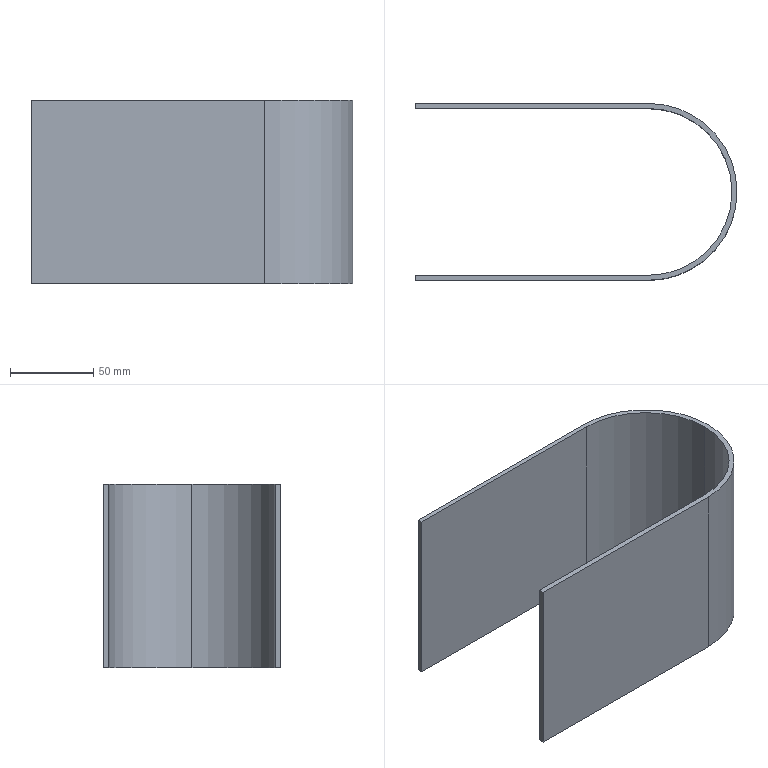Part | STEP file | 1 solid | 12 faces | box 193 x 106 x 110 mm | volume 145791 mm3 | plane 8 | cylinder 4 | commonest cylinder face diameters 100 x2 106 x2
STEP:
#1=CARTESIAN_POINT('',(0.,0.,0.));
#2=DIRECTION('',(0.,0.,1.));
#3=DIRECTION('',(1.,0.,0.));
#4=AXIS2_PLACEMENT_3D('',#1,#2,#3);
#5=CARTESIAN_POINT('',(27.634,-77.901,0.));
#6=VERTEX_POINT('',#5);
#7=CARTESIAN_POINT('',(80.634,-24.901,0.));
#8=VERTEX_POINT('',#7);
#9=CARTESIAN_POINT('',(27.634,-24.901,0.));
#10=DIRECTION('',(0.,0.,1.));
#11=DIRECTION('',(1.,0.,0.));
#12=AXIS2_PLACEMENT_3D('',#9,#10,#11);
#13=CIRCLE('',#12,53.);
#14=CARTESIAN_POINT('',(27.634,-24.901,0.));
#15=DIRECTION('',(0.,0.,1.));
#16=DIRECTION('',(1.,0.,0.));
#17=AXIS2_PLACEMENT_3D('',#14,#15,#16);
#18=CYLINDRICAL_SURFACE('',#17,53.);
#19=CARTESIAN_POINT('',(0.,0.));
#20=DIRECTION('',(1.,0.));
#21=VECTOR('',#20,1.);
#22=LINE('',#19,#21);
#23=(GEOMETRIC_REPRESENTATION_CONTEXT(2)PARAMETRIC_REPRESENTATION_CONTEXT()REPRESENTATION_CONTEXT('',''));
#24=DEFINITIONAL_REPRESENTATION('',(#22),#23);
#25=PCURVE('',#18,#24);
#26=CARTESIAN_POINT('',(-12.03,-24.901,0.));
#27=DIRECTION('',(0.,0.,1.));
#28=DIRECTION('',(1.,0.,0.));
#29=AXIS2_PLACEMENT_3D('',#26,#27,#28);
#30=PLANE('',#29);
#31=CARTESIAN_POINT('',(39.665,0.));
#32=DIRECTION('',(1.,0.));
#33=AXIS2_PLACEMENT_2D('',#31,#32);
#34=CIRCLE('',#33,53.);
#35=(GEOMETRIC_REPRESENTATION_CONTEXT(2)PARAMETRIC_REPRESENTATION_CONTEXT()REPRESENTATION_CONTEXT('',''));
#36=DEFINITIONAL_REPRESENTATION('',(#34),#35);
#37=PCURVE('',#30,#36);
#38=SURFACE_CURVE('',#13,(#25,#37),.PCURVE_S1.);
#39=EDGE_CURVE('',#6,#8,#38,.T.);
#40=ORIENTED_EDGE('',*,*,#39,.T.);
#41=CARTESIAN_POINT('',(80.634,-24.901,110.));
#42=VERTEX_POINT('',#41);
#43=CARTESIAN_POINT('',(80.634,-24.901,0.));
#44=DIRECTION('',(0.,0.,1.));
#45=VECTOR('',#44,1.);
#46=LINE('',#43,#45);
#47=CARTESIAN_POINT('',(6.283,0.));
#48=DIRECTION('',(0.,1.));
#49=VECTOR('',#48,1.);
#50=LINE('',#47,#49);
#51=(GEOMETRIC_REPRESENTATION_CONTEXT(2)PARAMETRIC_REPRESENTATION_CONTEXT()REPRESENTATION_CONTEXT('',''));
#52=DEFINITIONAL_REPRESENTATION('',(#50),#51);
#53=PCURVE('',#18,#52);
#54=CARTESIAN_POINT('',(27.634,-24.901,0.));
#55=DIRECTION('',(0.,0.,1.));
#56=DIRECTION('',(1.,0.,0.));
#57=AXIS2_PLACEMENT_3D('',#54,#55,#56);
#58=CYLINDRICAL_SURFACE('',#57,53.);
#59=CARTESIAN_POINT('',(0.,0.));
#60=DIRECTION('',(0.,1.));
#61=VECTOR('',#60,1.);
#62=LINE('',#59,#61);
#63=(GEOMETRIC_REPRESENTATION_CONTEXT(2)PARAMETRIC_REPRESENTATION_CONTEXT()REPRESENTATION_CONTEXT('',''));
#64=DEFINITIONAL_REPRESENTATION('',(#62),#63);
#65=PCURVE('',#58,#64);
#66=SURFACE_CURVE('',#46,(#53,#65),.PCURVE_S1.);
#67=EDGE_CURVE('',#8,#42,#66,.T.);
#68=ORIENTED_EDGE('',*,*,#67,.T.);
#69=CARTESIAN_POINT('',(27.634,-77.901,110.));
#70=VERTEX_POINT('',#69);
#71=CARTESIAN_POINT('',(27.634,-24.901,110.));
#72=DIRECTION('',(0.,0.,-1.));
#73=DIRECTION('',(1.,0.,0.));
#74=AXIS2_PLACEMENT_3D('',#71,#72,#73);
#75=CIRCLE('',#74,53.);
#76=CARTESIAN_POINT('',(6.283,110.));
#77=DIRECTION('',(-1.,0.));
#78=VECTOR('',#77,1.);
#79=LINE('',#76,#78);
#80=(GEOMETRIC_REPRESENTATION_CONTEXT(2)PARAMETRIC_REPRESENTATION_CONTEXT()REPRESENTATION_CONTEXT('',''));
#81=DEFINITIONAL_REPRESENTATION('',(#79),#80);
#82=PCURVE('',#18,#81);
#83=CARTESIAN_POINT('',(-12.03,-24.901,110.));
#84=DIRECTION('',(0.,0.,1.));
#85=DIRECTION('',(1.,0.,0.));
#86=AXIS2_PLACEMENT_3D('',#83,#84,#85);
#87=PLANE('',#86);
#88=CARTESIAN_POINT('',(92.665,0.));
#89=CARTESIAN_POINT('',(92.665,-91.799));
#90=CARTESIAN_POINT('',(13.165,-45.899));
#91=CARTESIAN_POINT('',(-66.335,0.));
#92=CARTESIAN_POINT('',(13.165,45.899));
#93=CARTESIAN_POINT('',(92.665,91.799));
#94=CARTESIAN_POINT('',(92.665,0.));
#95=(BOUNDED_CURVE()B_SPLINE_CURVE(2,(#88,#89,#90,#91,#92,#93,#94),.UNSPECIFIED.,.T.,.F.)B_SPLINE_CURVE_WITH_KNOTS((1,2,2,2,2,1),(-2.094,0.,2.094,4.189,6.283,8.378),.UNSPECIFIED.)CURVE()GEOMETRIC_REPRESENTATION_ITEM()RATIONAL_B_SPLINE_CURVE((1.,0.5,1.,0.5,1.,0.5,1.))REPRESENTATION_ITEM(''));
#96=(GEOMETRIC_REPRESENTATION_CONTEXT(2)PARAMETRIC_REPRESENTATION_CONTEXT()REPRESENTATION_CONTEXT('',''));
#97=DEFINITIONAL_REPRESENTATION('',(#95),#96);
#98=PCURVE('',#87,#97);
#99=SURFACE_CURVE('',#75,(#82,#98),.PCURVE_S1.);
#100=EDGE_CURVE('',#42,#70,#99,.T.);
#101=ORIENTED_EDGE('',*,*,#100,.T.);
#102=CARTESIAN_POINT('',(27.634,-77.901,0.));
#103=DIRECTION('',(0.,0.,-1.));
#104=VECTOR('',#103,1.);
#105=LINE('',#102,#104);
#106=CARTESIAN_POINT('',(4.712,0.));
#107=DIRECTION('',(0.,-1.));
#108=VECTOR('',#107,1.);
#109=LINE('',#106,#108);
#110=(GEOMETRIC_REPRESENTATION_CONTEXT(2)PARAMETRIC_REPRESENTATION_CONTEXT()REPRESENTATION_CONTEXT('',''));
#111=DEFINITIONAL_REPRESENTATION('',(#109),#110);
#112=PCURVE('',#18,#111);
#113=CARTESIAN_POINT('',(-112.366,-77.901,0.));
#114=DIRECTION('',(0.,-1.,0.));
#115=DIRECTION('',(1.,0.,0.));
#116=AXIS2_PLACEMENT_3D('',#113,#114,#115);
#117=PLANE('',#116);
#118=CARTESIAN_POINT('',(140.,0.));
#119=DIRECTION('',(0.,-1.));
#120=VECTOR('',#119,1.);
#121=LINE('',#118,#120);
#122=(GEOMETRIC_REPRESENTATION_CONTEXT(2)PARAMETRIC_REPRESENTATION_CONTEXT()REPRESENTATION_CONTEXT('',''));
#123=DEFINITIONAL_REPRESENTATION('',(#121),#122);
#124=PCURVE('',#117,#123);
#125=SURFACE_CURVE('',#105,(#112,#124),.PCURVE_S1.);
#126=EDGE_CURVE('',#70,#6,#125,.T.);
#127=ORIENTED_EDGE('',*,*,#126,.T.);
#128=EDGE_LOOP('',(#40,#68,#101,#127));
#129=FACE_BOUND('',#128,.T.);
#130=ADVANCED_FACE('',(#129),#18,.T.);
#131=CARTESIAN_POINT('',(27.634,25.099,0.));
#132=VERTEX_POINT('',#131);
#133=CARTESIAN_POINT('',(27.634,25.099,110.));
#134=VERTEX_POINT('',#133);
#135=CARTESIAN_POINT('',(27.634,25.099,0.));
#136=DIRECTION('',(0.,0.,1.));
#137=VECTOR('',#136,1.);
#138=LINE('',#135,#137);
#139=CARTESIAN_POINT('',(27.634,-24.901,0.));
#140=DIRECTION('',(0.,0.,1.));
#141=DIRECTION('',(1.,0.,0.));
#142=AXIS2_PLACEMENT_3D('',#139,#140,#141);
#143=CYLINDRICAL_SURFACE('',#142,50.);
#144=CARTESIAN_POINT('',(1.571,0.));
#145=DIRECTION('',(0.,1.));
#146=VECTOR('',#145,1.);
#147=LINE('',#144,#146);
#148=(GEOMETRIC_REPRESENTATION_CONTEXT(2)PARAMETRIC_REPRESENTATION_CONTEXT()REPRESENTATION_CONTEXT('',''));
#149=DEFINITIONAL_REPRESENTATION('',(#147),#148);
#150=PCURVE('',#143,#149);
#151=CARTESIAN_POINT('',(-112.366,25.099,0.));
#152=DIRECTION('',(0.,-1.,0.));
#153=DIRECTION('',(0.,0.,-1.));
#154=AXIS2_PLACEMENT_3D('',#151,#152,#153);
#155=PLANE('',#154);
#156=CARTESIAN_POINT('',(0.,140.));
#157=DIRECTION('',(-1.,0.));
#158=VECTOR('',#157,1.);
#159=LINE('',#156,#158);
#160=(GEOMETRIC_REPRESENTATION_CONTEXT(2)PARAMETRIC_REPRESENTATION_CONTEXT()REPRESENTATION_CONTEXT('',''));
#161=DEFINITIONAL_REPRESENTATION('',(#159),#160);
#162=PCURVE('',#155,#161);
#163=SURFACE_CURVE('',#138,(#150,#162),.PCURVE_S1.);
#164=EDGE_CURVE('',#132,#134,#163,.T.);
#165=ORIENTED_EDGE('',*,*,#164,.T.);
#166=CARTESIAN_POINT('',(77.634,-24.901,110.));
#167=VERTEX_POINT('',#166);
#168=CARTESIAN_POINT('',(27.634,-24.901,110.));
#169=DIRECTION('',(0.,0.,-1.));
#170=DIRECTION('',(1.,0.,0.));
#171=AXIS2_PLACEMENT_3D('',#168,#169,#170);
#172=CIRCLE('',#171,50.);
#173=CARTESIAN_POINT('',(6.283,110.));
#174=DIRECTION('',(-1.,0.));
#175=VECTOR('',#174,1.);
#176=LINE('',#173,#175);
#177=(GEOMETRIC_REPRESENTATION_CONTEXT(2)PARAMETRIC_REPRESENTATION_CONTEXT()REPRESENTATION_CONTEXT('',''));
#178=DEFINITIONAL_REPRESENTATION('',(#176),#177);
#179=PCURVE('',#143,#178);
#180=CARTESIAN_POINT('',(89.665,0.));
#181=CARTESIAN_POINT('',(89.665,-86.603));
#182=CARTESIAN_POINT('',(14.665,-43.301));
#183=CARTESIAN_POINT('',(-60.335,0.));
#184=CARTESIAN_POINT('',(14.665,43.301));
#185=CARTESIAN_POINT('',(89.665,86.603));
#186=CARTESIAN_POINT('',(89.665,0.));
#187=(BOUNDED_CURVE()B_SPLINE_CURVE(2,(#180,#181,#182,#183,#184,#185,#186),.UNSPECIFIED.,.T.,.F.)B_SPLINE_CURVE_WITH_KNOTS((1,2,2,2,2,1),(-2.094,0.,2.094,4.189,6.283,8.378),.UNSPECIFIED.)CURVE()GEOMETRIC_REPRESENTATION_ITEM()RATIONAL_B_SPLINE_CURVE((1.,0.5,1.,0.5,1.,0.5,1.))REPRESENTATION_ITEM(''));
#188=(GEOMETRIC_REPRESENTATION_CONTEXT(2)PARAMETRIC_REPRESENTATION_CONTEXT()REPRESENTATION_CONTEXT('',''));
#189=DEFINITIONAL_REPRESENTATION('',(#187),#188);
#190=PCURVE('',#87,#189);
#191=SURFACE_CURVE('',#172,(#179,#190),.PCURVE_S1.);
#192=EDGE_CURVE('',#134,#167,#191,.T.);
#193=ORIENTED_EDGE('',*,*,#192,.T.);
#194=CARTESIAN_POINT('',(77.634,-24.901,0.));
#195=VERTEX_POINT('',#194);
#196=CARTESIAN_POINT('',(77.634,-24.901,0.));
#197=DIRECTION('',(0.,0.,1.));
#198=VECTOR('',#197,1.);
#199=LINE('',#196,#198);
#200=CARTESIAN_POINT('',(0.,0.));
#201=DIRECTION('',(0.,1.));
#202=VECTOR('',#201,1.);
#203=LINE('',#200,#202);
#204=(GEOMETRIC_REPRESENTATION_CONTEXT(2)PARAMETRIC_REPRESENTATION_CONTEXT()REPRESENTATION_CONTEXT('',''));
#205=DEFINITIONAL_REPRESENTATION('',(#203),#204);
#206=PCURVE('',#143,#205);
#207=CARTESIAN_POINT('',(27.634,-24.901,0.));
#208=DIRECTION('',(0.,0.,1.));
#209=DIRECTION('',(1.,0.,0.));
#210=AXIS2_PLACEMENT_3D('',#207,#208,#209);
#211=CYLINDRICAL_SURFACE('',#210,50.);
#212=CARTESIAN_POINT('',(6.283,0.));
#213=DIRECTION('',(0.,1.));
#214=VECTOR('',#213,1.);
#215=LINE('',#212,#214);
#216=(GEOMETRIC_REPRESENTATION_CONTEXT(2)PARAMETRIC_REPRESENTATION_CONTEXT()REPRESENTATION_CONTEXT('',''));
#217=DEFINITIONAL_REPRESENTATION('',(#215),#216);
#218=PCURVE('',#211,#217);
#219=SURFACE_CURVE('',#199,(#206,#218),.PCURVE_S1.);
#220=EDGE_CURVE('',#195,#167,#219,.T.);
#221=ORIENTED_EDGE('',*,*,#220,.F.);
#222=CARTESIAN_POINT('',(27.634,-24.901,0.));
#223=DIRECTION('',(0.,0.,-1.));
#224=DIRECTION('',(1.,0.,0.));
#225=AXIS2_PLACEMENT_3D('',#222,#223,#224);
#226=CIRCLE('',#225,50.);
#227=CARTESIAN_POINT('',(6.283,0.));
#228=DIRECTION('',(-1.,0.));
#229=VECTOR('',#228,1.);
#230=LINE('',#227,#229);
#231=(GEOMETRIC_REPRESENTATION_CONTEXT(2)PARAMETRIC_REPRESENTATION_CONTEXT()REPRESENTATION_CONTEXT('',''));
#232=DEFINITIONAL_REPRESENTATION('',(#230),#231);
#233=PCURVE('',#143,#232);
#234=CARTESIAN_POINT('',(89.665,0.));
#235=CARTESIAN_POINT('',(89.665,-86.603));
#236=CARTESIAN_POINT('',(14.665,-43.301));
#237=CARTESIAN_POINT('',(-60.335,0.));
#238=CARTESIAN_POINT('',(14.665,43.301));
#239=CARTESIAN_POINT('',(89.665,86.603));
#240=CARTESIAN_POINT('',(89.665,0.));
#241=(BOUNDED_CURVE()B_SPLINE_CURVE(2,(#234,#235,#236,#237,#238,#239,#240),.UNSPECIFIED.,.T.,.F.)B_SPLINE_CURVE_WITH_KNOTS((1,2,2,2,2,1),(-2.094,0.,2.094,4.189,6.283,8.378),.UNSPECIFIED.)CURVE()GEOMETRIC_REPRESENTATION_ITEM()RATIONAL_B_SPLINE_CURVE((1.,0.5,1.,0.5,1.,0.5,1.))REPRESENTATION_ITEM(''));
#242=(GEOMETRIC_REPRESENTATION_CONTEXT(2)PARAMETRIC_REPRESENTATION_CONTEXT()REPRESENTATION_CONTEXT('',''));
#243=DEFINITIONAL_REPRESENTATION('',(#241),#242);
#244=PCURVE('',#30,#243);
#245=SURFACE_CURVE('',#226,(#233,#244),.PCURVE_S1.);
#246=EDGE_CURVE('',#132,#195,#245,.T.);
#247=ORIENTED_EDGE('',*,*,#246,.F.);
#248=EDGE_LOOP('',(#165,#193,#221,#247));
#249=FACE_BOUND('',#248,.F.);
#250=ADVANCED_FACE('',(#249),#143,.F.);
#251=ORIENTED_EDGE('',*,*,#67,.F.);
#252=CARTESIAN_POINT('',(27.634,28.099,0.));
#253=VERTEX_POINT('',#252);
#254=CARTESIAN_POINT('',(27.634,-24.901,0.));
#255=DIRECTION('',(0.,0.,1.));
#256=DIRECTION('',(1.,0.,0.));
#257=AXIS2_PLACEMENT_3D('',#254,#255,#256);
#258=CIRCLE('',#257,53.);
#259=CARTESIAN_POINT('',(0.,0.));
#260=DIRECTION('',(1.,0.));
#261=VECTOR('',#260,1.);
#262=LINE('',#259,#261);
#263=(GEOMETRIC_REPRESENTATION_CONTEXT(2)PARAMETRIC_REPRESENTATION_CONTEXT()REPRESENTATION_CONTEXT('',''));
#264=DEFINITIONAL_REPRESENTATION('',(#262),#263);
#265=PCURVE('',#58,#264);
#266=CARTESIAN_POINT('',(39.665,0.));
#267=DIRECTION('',(1.,0.));
#268=AXIS2_PLACEMENT_2D('',#266,#267);
#269=CIRCLE('',#268,53.);
#270=(GEOMETRIC_REPRESENTATION_CONTEXT(2)PARAMETRIC_REPRESENTATION_CONTEXT()REPRESENTATION_CONTEXT('',''));
#271=DEFINITIONAL_REPRESENTATION('',(#269),#270);
#272=PCURVE('',#30,#271);
#273=SURFACE_CURVE('',#258,(#265,#272),.PCURVE_S1.);
#274=EDGE_CURVE('',#8,#253,#273,.T.);
#275=ORIENTED_EDGE('',*,*,#274,.T.);
#276=CARTESIAN_POINT('',(27.634,28.099,110.));
#277=VERTEX_POINT('',#276);
#278=CARTESIAN_POINT('',(27.634,28.099,0.));
#279=DIRECTION('',(0.,0.,1.));
#280=VECTOR('',#279,1.);
#281=LINE('',#278,#280);
#282=CARTESIAN_POINT('',(1.571,0.));
#283=DIRECTION('',(0.,1.));
#284=VECTOR('',#283,1.);
#285=LINE('',#282,#284);
#286=(GEOMETRIC_REPRESENTATION_CONTEXT(2)PARAMETRIC_REPRESENTATION_CONTEXT()REPRESENTATION_CONTEXT('',''));
#287=DEFINITIONAL_REPRESENTATION('',(#285),#286);
#288=PCURVE('',#58,#287);
#289=CARTESIAN_POINT('',(27.634,28.099,0.));
#290=DIRECTION('',(0.,1.,0.));
#291=DIRECTION('',(-1.,0.,0.));
#292=AXIS2_PLACEMENT_3D('',#289,#290,#291);
#293=PLANE('',#292);
#294=CARTESIAN_POINT('',(0.,0.));
#295=DIRECTION('',(0.,1.));
#296=VECTOR('',#295,1.);
#297=LINE('',#294,#296);
#298=(GEOMETRIC_REPRESENTATION_CONTEXT(2)PARAMETRIC_REPRESENTATION_CONTEXT()REPRESENTATION_CONTEXT('',''));
#299=DEFINITIONAL_REPRESENTATION('',(#297),#298);
#300=PCURVE('',#293,#299);
#301=SURFACE_CURVE('',#281,(#288,#300),.PCURVE_S1.);
#302=EDGE_CURVE('',#253,#277,#301,.T.);
#303=ORIENTED_EDGE('',*,*,#302,.T.);
#304=CARTESIAN_POINT('',(27.634,-24.901,110.));
#305=DIRECTION('',(0.,0.,-1.));
#306=DIRECTION('',(1.,0.,0.));
#307=AXIS2_PLACEMENT_3D('',#304,#305,#306);
#308=CIRCLE('',#307,53.);
#309=CARTESIAN_POINT('',(6.283,110.));
#310=DIRECTION('',(-1.,0.));
#311=VECTOR('',#310,1.);
#312=LINE('',#309,#311);
#313=(GEOMETRIC_REPRESENTATION_CONTEXT(2)PARAMETRIC_REPRESENTATION_CONTEXT()REPRESENTATION_CONTEXT('',''));
#314=DEFINITIONAL_REPRESENTATION('',(#312),#313);
#315=PCURVE('',#58,#314);
#316=CARTESIAN_POINT('',(92.665,0.));
#317=CARTESIAN_POINT('',(92.665,-91.799));
#318=CARTESIAN_POINT('',(13.165,-45.899));
#319=CARTESIAN_POINT('',(-66.335,0.));
#320=CARTESIAN_POINT('',(13.165,45.899));
#321=CARTESIAN_POINT('',(92.665,91.799));
#322=CARTESIAN_POINT('',(92.665,0.));
#323=(BOUNDED_CURVE()B_SPLINE_CURVE(2,(#316,#317,#318,#319,#320,#321,#322),.UNSPECIFIED.,.T.,.F.)B_SPLINE_CURVE_WITH_KNOTS((1,2,2,2,2,1),(-2.094,0.,2.094,4.189,6.283,8.378),.UNSPECIFIED.)CURVE()GEOMETRIC_REPRESENTATION_ITEM()RATIONAL_B_SPLINE_CURVE((1.,0.5,1.,0.5,1.,0.5,1.))REPRESENTATION_ITEM(''));
#324=(GEOMETRIC_REPRESENTATION_CONTEXT(2)PARAMETRIC_REPRESENTATION_CONTEXT()REPRESENTATION_CONTEXT('',''));
#325=DEFINITIONAL_REPRESENTATION('',(#323),#324);
#326=PCURVE('',#87,#325);
#327=SURFACE_CURVE('',#308,(#315,#326),.PCURVE_S1.);
#328=EDGE_CURVE('',#277,#42,#327,.T.);
#329=ORIENTED_EDGE('',*,*,#328,.T.);
#330=EDGE_LOOP('',(#251,#275,#303,#329));
#331=FACE_BOUND('',#330,.T.);
#332=ADVANCED_FACE('',(#331),#58,.T.);
#333=CARTESIAN_POINT('',(-112.366,-77.901,110.));
#334=VERTEX_POINT('',#333);
#335=CARTESIAN_POINT('',(-112.366,-77.901,110.));
#336=DIRECTION('',(-1.,0.,0.));
#337=VECTOR('',#336,1.);
#338=LINE('',#335,#337);
#339=CARTESIAN_POINT('',(0.,110.));
#340=DIRECTION('',(-1.,0.));
#341=VECTOR('',#340,1.);
#342=LINE('',#339,#341);
#343=(GEOMETRIC_REPRESENTATION_CONTEXT(2)PARAMETRIC_REPRESENTATION_CONTEXT()REPRESENTATION_CONTEXT('',''));
#344=DEFINITIONAL_REPRESENTATION('',(#342),#343);
#345=PCURVE('',#117,#344);
#346=CARTESIAN_POINT('',(-100.335,-53.));
#347=DIRECTION('',(-1.,0.));
#348=VECTOR('',#347,1.);
#349=LINE('',#346,#348);
#350=(GEOMETRIC_REPRESENTATION_CONTEXT(2)PARAMETRIC_REPRESENTATION_CONTEXT()REPRESENTATION_CONTEXT('',''));
#351=DEFINITIONAL_REPRESENTATION('',(#349),#350);
#352=PCURVE('',#87,#351);
#353=SURFACE_CURVE('',#338,(#345,#352),.PCURVE_S1.);
#354=EDGE_CURVE('',#70,#334,#353,.T.);
#355=ORIENTED_EDGE('',*,*,#354,.T.);
#356=CARTESIAN_POINT('',(-112.366,-77.901,0.));
#357=VERTEX_POINT('',#356);
#358=CARTESIAN_POINT('',(-112.366,-77.901,0.));
#359=DIRECTION('',(0.,0.,-1.));
#360=VECTOR('',#359,1.);
#361=LINE('',#358,#360);
#362=CARTESIAN_POINT('',(0.,0.));
#363=DIRECTION('',(0.,-1.));
#364=VECTOR('',#363,1.);
#365=LINE('',#362,#364);
#366=(GEOMETRIC_REPRESENTATION_CONTEXT(2)PARAMETRIC_REPRESENTATION_CONTEXT()REPRESENTATION_CONTEXT('',''));
#367=DEFINITIONAL_REPRESENTATION('',(#365),#366);
#368=PCURVE('',#117,#367);
#369=CARTESIAN_POINT('',(-112.366,-74.901,0.));
#370=DIRECTION('',(-1.,0.,0.));
#371=DIRECTION('',(0.,0.,1.));
#372=AXIS2_PLACEMENT_3D('',#369,#370,#371);
#373=PLANE('',#372);
#374=CARTESIAN_POINT('',(0.,-3.));
#375=DIRECTION('',(-1.,0.));
#376=VECTOR('',#375,1.);
#377=LINE('',#374,#376);
#378=(GEOMETRIC_REPRESENTATION_CONTEXT(2)PARAMETRIC_REPRESENTATION_CONTEXT()REPRESENTATION_CONTEXT('',''));
#379=DEFINITIONAL_REPRESENTATION('',(#377),#378);
#380=PCURVE('',#373,#379);
#381=SURFACE_CURVE('',#361,(#368,#380),.PCURVE_S1.);
#382=EDGE_CURVE('',#334,#357,#381,.T.);
#383=ORIENTED_EDGE('',*,*,#382,.T.);
#384=CARTESIAN_POINT('',(-112.366,-77.901,0.));
#385=DIRECTION('',(1.,0.,0.));
#386=VECTOR('',#385,1.);
#387=LINE('',#384,#386);
#388=CARTESIAN_POINT('',(0.,0.));
#389=DIRECTION('',(1.,0.));
#390=VECTOR('',#389,1.);
#391=LINE('',#388,#390);
#392=(GEOMETRIC_REPRESENTATION_CONTEXT(2)PARAMETRIC_REPRESENTATION_CONTEXT()REPRESENTATION_CONTEXT('',''));
#393=DEFINITIONAL_REPRESENTATION('',(#391),#392);
#394=PCURVE('',#117,#393);
#395=CARTESIAN_POINT('',(-100.335,-53.));
#396=DIRECTION('',(1.,0.));
#397=VECTOR('',#396,1.);
#398=LINE('',#395,#397);
#399=(GEOMETRIC_REPRESENTATION_CONTEXT(2)PARAMETRIC_REPRESENTATION_CONTEXT()REPRESENTATION_CONTEXT('',''));
#400=DEFINITIONAL_REPRESENTATION('',(#398),#399);
#401=PCURVE('',#30,#400);
#402=SURFACE_CURVE('',#387,(#394,#401),.PCURVE_S1.);
#403=EDGE_CURVE('',#357,#6,#402,.T.);
#404=ORIENTED_EDGE('',*,*,#403,.T.);
#405=ORIENTED_EDGE('',*,*,#126,.F.);
#406=EDGE_LOOP('',(#355,#383,#404,#405));
#407=FACE_BOUND('',#406,.T.);
#408=ADVANCED_FACE('',(#407),#117,.T.);
#409=CARTESIAN_POINT('',(-112.366,28.099,110.));
#410=VERTEX_POINT('',#409);
#411=CARTESIAN_POINT('',(-12.03,28.099,110.));
#412=DIRECTION('',(-1.,0.,0.));
#413=VECTOR('',#412,1.);
#414=LINE('',#411,#413);
#415=CARTESIAN_POINT('',(0.,53.));
#416=DIRECTION('',(-1.,0.));
#417=VECTOR('',#416,1.);
#418=LINE('',#415,#417);
#419=(GEOMETRIC_REPRESENTATION_CONTEXT(2)PARAMETRIC_REPRESENTATION_CONTEXT()REPRESENTATION_CONTEXT('',''));
#420=DEFINITIONAL_REPRESENTATION('',(#418),#419);
#421=PCURVE('',#87,#420);
#422=CARTESIAN_POINT('',(39.665,110.));
#423=DIRECTION('',(1.,0.));
#424=VECTOR('',#423,1.);
#425=LINE('',#422,#424);
#426=(GEOMETRIC_REPRESENTATION_CONTEXT(2)PARAMETRIC_REPRESENTATION_CONTEXT()REPRESENTATION_CONTEXT('',''));
#427=DEFINITIONAL_REPRESENTATION('',(#425),#426);
#428=PCURVE('',#293,#427);
#429=SURFACE_CURVE('',#414,(#421,#428),.PCURVE_S1.);
#430=EDGE_CURVE('',#277,#410,#429,.T.);
#431=ORIENTED_EDGE('',*,*,#430,.T.);
#432=CARTESIAN_POINT('',(-112.366,25.099,110.));
#433=VERTEX_POINT('',#432);
#434=CARTESIAN_POINT('',(-112.366,-24.901,110.));
#435=DIRECTION('',(0.,-1.,0.));
#436=VECTOR('',#435,1.);
#437=LINE('',#434,#436);
#438=CARTESIAN_POINT('',(-100.335,0.));
#439=DIRECTION('',(0.,-1.));
#440=VECTOR('',#439,1.);
#441=LINE('',#438,#440);
#442=(GEOMETRIC_REPRESENTATION_CONTEXT(2)PARAMETRIC_REPRESENTATION_CONTEXT()REPRESENTATION_CONTEXT('',''));
#443=DEFINITIONAL_REPRESENTATION('',(#441),#442);
#444=PCURVE('',#87,#443);
#445=CARTESIAN_POINT('',(-112.366,28.099,0.));
#446=DIRECTION('',(-1.,0.,0.));
#447=DIRECTION('',(0.,0.,1.));
#448=AXIS2_PLACEMENT_3D('',#445,#446,#447);
#449=PLANE('',#448);
#450=CARTESIAN_POINT('',(110.,-53.));
#451=DIRECTION('',(0.,-1.));
#452=VECTOR('',#451,1.);
#453=LINE('',#450,#452);
#454=(GEOMETRIC_REPRESENTATION_CONTEXT(2)PARAMETRIC_REPRESENTATION_CONTEXT()REPRESENTATION_CONTEXT('',''));
#455=DEFINITIONAL_REPRESENTATION('',(#453),#454);
#456=PCURVE('',#449,#455);
#457=SURFACE_CURVE('',#437,(#444,#456),.PCURVE_S1.);
#458=EDGE_CURVE('',#410,#433,#457,.T.);
#459=ORIENTED_EDGE('',*,*,#458,.T.);
#460=CARTESIAN_POINT('',(-12.03,25.099,110.));
#461=DIRECTION('',(1.,0.,0.));
#462=VECTOR('',#461,1.);
#463=LINE('',#460,#462);
#464=CARTESIAN_POINT('',(0.,50.));
#465=DIRECTION('',(1.,0.));
#466=VECTOR('',#465,1.);
#467=LINE('',#464,#466);
#468=(GEOMETRIC_REPRESENTATION_CONTEXT(2)PARAMETRIC_REPRESENTATION_CONTEXT()REPRESENTATION_CONTEXT('',''));
#469=DEFINITIONAL_REPRESENTATION('',(#467),#468);
#470=PCURVE('',#87,#469);
#471=CARTESIAN_POINT('',(-110.,100.335));
#472=DIRECTION('',(0.,1.));
#473=VECTOR('',#472,1.);
#474=LINE('',#471,#473);
#475=(GEOMETRIC_REPRESENTATION_CONTEXT(2)PARAMETRIC_REPRESENTATION_CONTEXT()REPRESENTATION_CONTEXT('',''));
#476=DEFINITIONAL_REPRESENTATION('',(#474),#475);
#477=PCURVE('',#155,#476);
#478=SURFACE_CURVE('',#463,(#470,#477),.PCURVE_S1.);
#479=EDGE_CURVE('',#433,#134,#478,.T.);
#480=ORIENTED_EDGE('',*,*,#479,.T.);
#481=ORIENTED_EDGE('',*,*,#192,.T.);
#482=CARTESIAN_POINT('',(27.634,-74.901,110.));
#483=VERTEX_POINT('',#482);
#484=CARTESIAN_POINT('',(27.634,-24.901,110.));
#485=DIRECTION('',(0.,0.,-1.));
#486=DIRECTION('',(1.,0.,0.));
#487=AXIS2_PLACEMENT_3D('',#484,#485,#486);
#488=CIRCLE('',#487,50.);
#489=CARTESIAN_POINT('',(89.665,0.));
#490=CARTESIAN_POINT('',(89.665,-86.603));
#491=CARTESIAN_POINT('',(14.665,-43.301));
#492=CARTESIAN_POINT('',(-60.335,0.));
#493=CARTESIAN_POINT('',(14.665,43.301));
#494=CARTESIAN_POINT('',(89.665,86.603));
#495=CARTESIAN_POINT('',(89.665,0.));
#496=(BOUNDED_CURVE()B_SPLINE_CURVE(2,(#489,#490,#491,#492,#493,#494,#495),.UNSPECIFIED.,.T.,.F.)B_SPLINE_CURVE_WITH_KNOTS((1,2,2,2,2,1),(-2.094,0.,2.094,4.189,6.283,8.378),.UNSPECIFIED.)CURVE()GEOMETRIC_REPRESENTATION_ITEM()RATIONAL_B_SPLINE_CURVE((1.,0.5,1.,0.5,1.,0.5,1.))REPRESENTATION_ITEM(''));
#497=(GEOMETRIC_REPRESENTATION_CONTEXT(2)PARAMETRIC_REPRESENTATION_CONTEXT()REPRESENTATION_CONTEXT('',''));
#498=DEFINITIONAL_REPRESENTATION('',(#496),#497);
#499=PCURVE('',#87,#498);
#500=CARTESIAN_POINT('',(6.283,110.));
#501=DIRECTION('',(-1.,0.));
#502=VECTOR('',#501,1.);
#503=LINE('',#500,#502);
#504=(GEOMETRIC_REPRESENTATION_CONTEXT(2)PARAMETRIC_REPRESENTATION_CONTEXT()REPRESENTATION_CONTEXT('',''));
#505=DEFINITIONAL_REPRESENTATION('',(#503),#504);
#506=PCURVE('',#211,#505);
#507=SURFACE_CURVE('',#488,(#499,#506),.PCURVE_S1.);
#508=EDGE_CURVE('',#167,#483,#507,.T.);
#509=ORIENTED_EDGE('',*,*,#508,.T.);
#510=CARTESIAN_POINT('',(-112.366,-74.901,110.));
#511=VERTEX_POINT('',#510);
#512=CARTESIAN_POINT('',(-12.03,-74.901,110.));
#513=DIRECTION('',(-1.,0.,0.));
#514=VECTOR('',#513,1.);
#515=LINE('',#512,#514);
#516=CARTESIAN_POINT('',(0.,-50.));
#517=DIRECTION('',(-1.,0.));
#518=VECTOR('',#517,1.);
#519=LINE('',#516,#518);
#520=(GEOMETRIC_REPRESENTATION_CONTEXT(2)PARAMETRIC_REPRESENTATION_CONTEXT()REPRESENTATION_CONTEXT('',''));
#521=DEFINITIONAL_REPRESENTATION('',(#519),#520);
#522=PCURVE('',#87,#521);
#523=CARTESIAN_POINT('',(27.634,-74.901,0.));
#524=DIRECTION('',(0.,1.,0.));
#525=DIRECTION('',(-1.,0.,0.));
#526=AXIS2_PLACEMENT_3D('',#523,#524,#525);
#527=PLANE('',#526);
#528=CARTESIAN_POINT('',(39.665,110.));
#529=DIRECTION('',(1.,0.));
#530=VECTOR('',#529,1.);
#531=LINE('',#528,#530);
#532=(GEOMETRIC_REPRESENTATION_CONTEXT(2)PARAMETRIC_REPRESENTATION_CONTEXT()REPRESENTATION_CONTEXT('',''));
#533=DEFINITIONAL_REPRESENTATION('',(#531),#532);
#534=PCURVE('',#527,#533);
#535=SURFACE_CURVE('',#515,(#522,#534),.PCURVE_S1.);
#536=EDGE_CURVE('',#483,#511,#535,.T.);
#537=ORIENTED_EDGE('',*,*,#536,.T.);
#538=CARTESIAN_POINT('',(-112.366,-24.901,110.));
#539=DIRECTION('',(0.,-1.,0.));
#540=VECTOR('',#539,1.);
#541=LINE('',#538,#540);
#542=CARTESIAN_POINT('',(-100.335,0.));
#543=DIRECTION('',(0.,-1.));
#544=VECTOR('',#543,1.);
#545=LINE('',#542,#544);
#546=(GEOMETRIC_REPRESENTATION_CONTEXT(2)PARAMETRIC_REPRESENTATION_CONTEXT()REPRESENTATION_CONTEXT('',''));
#547=DEFINITIONAL_REPRESENTATION('',(#545),#546);
#548=PCURVE('',#87,#547);
#549=CARTESIAN_POINT('',(110.,50.));
#550=DIRECTION('',(0.,-1.));
#551=VECTOR('',#550,1.);
#552=LINE('',#549,#551);
#553=(GEOMETRIC_REPRESENTATION_CONTEXT(2)PARAMETRIC_REPRESENTATION_CONTEXT()REPRESENTATION_CONTEXT('',''));
#554=DEFINITIONAL_REPRESENTATION('',(#552),#553);
#555=PCURVE('',#373,#554);
#556=SURFACE_CURVE('',#541,(#548,#555),.PCURVE_S1.);
#557=EDGE_CURVE('',#511,#334,#556,.T.);
#558=ORIENTED_EDGE('',*,*,#557,.T.);
#559=ORIENTED_EDGE('',*,*,#354,.F.);
#560=ORIENTED_EDGE('',*,*,#100,.F.);
#561=ORIENTED_EDGE('',*,*,#328,.F.);
#562=EDGE_LOOP('',(#431,#459,#480,#481,#509,#537,#558,#559,#560,#561));
#563=FACE_BOUND('',#562,.T.);
#564=ADVANCED_FACE('',(#563),#87,.T.);
#565=ORIENTED_EDGE('',*,*,#430,.F.);
#566=ORIENTED_EDGE('',*,*,#302,.F.);
#567=CARTESIAN_POINT('',(-112.366,28.099,0.));
#568=VERTEX_POINT('',#567);
#569=CARTESIAN_POINT('',(27.634,28.099,0.));
#570=DIRECTION('',(-1.,0.,0.));
#571=VECTOR('',#570,1.);
#572=LINE('',#569,#571);
#573=CARTESIAN_POINT('',(0.,0.));
#574=DIRECTION('',(1.,0.));
#575=VECTOR('',#574,1.);
#576=LINE('',#573,#575);
#577=(GEOMETRIC_REPRESENTATION_CONTEXT(2)PARAMETRIC_REPRESENTATION_CONTEXT()REPRESENTATION_CONTEXT('',''));
#578=DEFINITIONAL_REPRESENTATION('',(#576),#577);
#579=PCURVE('',#293,#578);
#580=CARTESIAN_POINT('',(39.665,53.));
#581=DIRECTION('',(-1.,0.));
#582=VECTOR('',#581,1.);
#583=LINE('',#580,#582);
#584=(GEOMETRIC_REPRESENTATION_CONTEXT(2)PARAMETRIC_REPRESENTATION_CONTEXT()REPRESENTATION_CONTEXT('',''));
#585=DEFINITIONAL_REPRESENTATION('',(#583),#584);
#586=PCURVE('',#30,#585);
#587=SURFACE_CURVE('',#572,(#579,#586),.PCURVE_S1.);
#588=EDGE_CURVE('',#253,#568,#587,.T.);
#589=ORIENTED_EDGE('',*,*,#588,.T.);
#590=CARTESIAN_POINT('',(-112.366,28.099,0.));
#591=DIRECTION('',(0.,0.,1.));
#592=VECTOR('',#591,1.);
#593=LINE('',#590,#592);
#594=CARTESIAN_POINT('',(140.,0.));
#595=DIRECTION('',(0.,1.));
#596=VECTOR('',#595,1.);
#597=LINE('',#594,#596);
#598=(GEOMETRIC_REPRESENTATION_CONTEXT(2)PARAMETRIC_REPRESENTATION_CONTEXT()REPRESENTATION_CONTEXT('',''));
#599=DEFINITIONAL_REPRESENTATION('',(#597),#598);
#600=PCURVE('',#293,#599);
#601=CARTESIAN_POINT('',(0.,0.));
#602=DIRECTION('',(1.,0.));
#603=VECTOR('',#602,1.);
#604=LINE('',#601,#603);
#605=(GEOMETRIC_REPRESENTATION_CONTEXT(2)PARAMETRIC_REPRESENTATION_CONTEXT()REPRESENTATION_CONTEXT('',''));
#606=DEFINITIONAL_REPRESENTATION('',(#604),#605);
#607=PCURVE('',#449,#606);
#608=SURFACE_CURVE('',#593,(#600,#607),.PCURVE_S1.);
#609=EDGE_CURVE('',#568,#410,#608,.T.);
#610=ORIENTED_EDGE('',*,*,#609,.T.);
#611=EDGE_LOOP('',(#565,#566,#589,#610));
#612=FACE_BOUND('',#611,.T.);
#613=ADVANCED_FACE('',(#612),#293,.T.);
#614=CARTESIAN_POINT('',(-112.366,25.099,0.));
#615=VERTEX_POINT('',#614);
#616=CARTESIAN_POINT('',(-112.366,-24.901,0.));
#617=DIRECTION('',(0.,-1.,0.));
#618=VECTOR('',#617,1.);
#619=LINE('',#616,#618);
#620=CARTESIAN_POINT('',(-100.335,0.));
#621=DIRECTION('',(0.,-1.));
#622=VECTOR('',#621,1.);
#623=LINE('',#620,#622);
#624=(GEOMETRIC_REPRESENTATION_CONTEXT(2)PARAMETRIC_REPRESENTATION_CONTEXT()REPRESENTATION_CONTEXT('',''));
#625=DEFINITIONAL_REPRESENTATION('',(#623),#624);
#626=PCURVE('',#30,#625);
#627=CARTESIAN_POINT('',(0.,-53.));
#628=DIRECTION('',(0.,-1.));
#629=VECTOR('',#628,1.);
#630=LINE('',#627,#629);
#631=(GEOMETRIC_REPRESENTATION_CONTEXT(2)PARAMETRIC_REPRESENTATION_CONTEXT()REPRESENTATION_CONTEXT('',''));
#632=DEFINITIONAL_REPRESENTATION('',(#630),#631);
#633=PCURVE('',#449,#632);
#634=SURFACE_CURVE('',#619,(#626,#633),.PCURVE_S1.);
#635=EDGE_CURVE('',#568,#615,#634,.T.);
#636=ORIENTED_EDGE('',*,*,#635,.F.);
#637=ORIENTED_EDGE('',*,*,#588,.F.);
#638=ORIENTED_EDGE('',*,*,#274,.F.);
#639=ORIENTED_EDGE('',*,*,#39,.F.);
#640=ORIENTED_EDGE('',*,*,#403,.F.);
#641=CARTESIAN_POINT('',(-112.366,-74.901,0.));
#642=VERTEX_POINT('',#641);
#643=CARTESIAN_POINT('',(-112.366,-24.901,0.));
#644=DIRECTION('',(0.,-1.,0.));
#645=VECTOR('',#644,1.);
#646=LINE('',#643,#645);
#647=CARTESIAN_POINT('',(-100.335,0.));
#648=DIRECTION('',(0.,-1.));
#649=VECTOR('',#648,1.);
#650=LINE('',#647,#649);
#651=(GEOMETRIC_REPRESENTATION_CONTEXT(2)PARAMETRIC_REPRESENTATION_CONTEXT()REPRESENTATION_CONTEXT('',''));
#652=DEFINITIONAL_REPRESENTATION('',(#650),#651);
#653=PCURVE('',#30,#652);
#654=CARTESIAN_POINT('',(0.,50.));
#655=DIRECTION('',(0.,-1.));
#656=VECTOR('',#655,1.);
#657=LINE('',#654,#656);
#658=(GEOMETRIC_REPRESENTATION_CONTEXT(2)PARAMETRIC_REPRESENTATION_CONTEXT()REPRESENTATION_CONTEXT('',''));
#659=DEFINITIONAL_REPRESENTATION('',(#657),#658);
#660=PCURVE('',#373,#659);
#661=SURFACE_CURVE('',#646,(#653,#660),.PCURVE_S1.);
#662=EDGE_CURVE('',#642,#357,#661,.T.);
#663=ORIENTED_EDGE('',*,*,#662,.F.);
#664=CARTESIAN_POINT('',(27.634,-74.901,0.));
#665=VERTEX_POINT('',#664);
#666=CARTESIAN_POINT('',(-12.03,-74.901,0.));
#667=DIRECTION('',(-1.,0.,0.));
#668=VECTOR('',#667,1.);
#669=LINE('',#666,#668);
#670=CARTESIAN_POINT('',(0.,-50.));
#671=DIRECTION('',(-1.,0.));
#672=VECTOR('',#671,1.);
#673=LINE('',#670,#672);
#674=(GEOMETRIC_REPRESENTATION_CONTEXT(2)PARAMETRIC_REPRESENTATION_CONTEXT()REPRESENTATION_CONTEXT('',''));
#675=DEFINITIONAL_REPRESENTATION('',(#673),#674);
#676=PCURVE('',#30,#675);
#677=CARTESIAN_POINT('',(39.665,0.));
#678=DIRECTION('',(1.,0.));
#679=VECTOR('',#678,1.);
#680=LINE('',#677,#679);
#681=(GEOMETRIC_REPRESENTATION_CONTEXT(2)PARAMETRIC_REPRESENTATION_CONTEXT()REPRESENTATION_CONTEXT('',''));
#682=DEFINITIONAL_REPRESENTATION('',(#680),#681);
#683=PCURVE('',#527,#682);
#684=SURFACE_CURVE('',#669,(#676,#683),.PCURVE_S1.);
#685=EDGE_CURVE('',#665,#642,#684,.T.);
#686=ORIENTED_EDGE('',*,*,#685,.F.);
#687=CARTESIAN_POINT('',(27.634,-24.901,0.));
#688=DIRECTION('',(0.,0.,-1.));
#689=DIRECTION('',(1.,0.,0.));
#690=AXIS2_PLACEMENT_3D('',#687,#688,#689);
#691=CIRCLE('',#690,50.);
#692=CARTESIAN_POINT('',(89.665,0.));
#693=CARTESIAN_POINT('',(89.665,-86.603));
#694=CARTESIAN_POINT('',(14.665,-43.301));
#695=CARTESIAN_POINT('',(-60.335,0.));
#696=CARTESIAN_POINT('',(14.665,43.301));
#697=CARTESIAN_POINT('',(89.665,86.603));
#698=CARTESIAN_POINT('',(89.665,0.));
#699=(BOUNDED_CURVE()B_SPLINE_CURVE(2,(#692,#693,#694,#695,#696,#697,#698),.UNSPECIFIED.,.T.,.F.)B_SPLINE_CURVE_WITH_KNOTS((1,2,2,2,2,1),(-2.094,0.,2.094,4.189,6.283,8.378),.UNSPECIFIED.)CURVE()GEOMETRIC_REPRESENTATION_ITEM()RATIONAL_B_SPLINE_CURVE((1.,0.5,1.,0.5,1.,0.5,1.))REPRESENTATION_ITEM(''));
#700=(GEOMETRIC_REPRESENTATION_CONTEXT(2)PARAMETRIC_REPRESENTATION_CONTEXT()REPRESENTATION_CONTEXT('',''));
#701=DEFINITIONAL_REPRESENTATION('',(#699),#700);
#702=PCURVE('',#30,#701);
#703=CARTESIAN_POINT('',(6.283,0.));
#704=DIRECTION('',(-1.,0.));
#705=VECTOR('',#704,1.);
#706=LINE('',#703,#705);
#707=(GEOMETRIC_REPRESENTATION_CONTEXT(2)PARAMETRIC_REPRESENTATION_CONTEXT()REPRESENTATION_CONTEXT('',''));
#708=DEFINITIONAL_REPRESENTATION('',(#706),#707);
#709=PCURVE('',#211,#708);
#710=SURFACE_CURVE('',#691,(#702,#709),.PCURVE_S1.);
#711=EDGE_CURVE('',#195,#665,#710,.T.);
#712=ORIENTED_EDGE('',*,*,#711,.F.);
#713=ORIENTED_EDGE('',*,*,#246,.F.);
#714=CARTESIAN_POINT('',(-12.03,25.099,0.));
#715=DIRECTION('',(1.,0.,0.));
#716=VECTOR('',#715,1.);
#717=LINE('',#714,#716);
#718=CARTESIAN_POINT('',(0.,50.));
#719=DIRECTION('',(1.,0.));
#720=VECTOR('',#719,1.);
#721=LINE('',#718,#720);
#722=(GEOMETRIC_REPRESENTATION_CONTEXT(2)PARAMETRIC_REPRESENTATION_CONTEXT()REPRESENTATION_CONTEXT('',''));
#723=DEFINITIONAL_REPRESENTATION('',(#721),#722);
#724=PCURVE('',#30,#723);
#725=CARTESIAN_POINT('',(0.,100.335));
#726=DIRECTION('',(0.,1.));
#727=VECTOR('',#726,1.);
#728=LINE('',#725,#727);
#729=(GEOMETRIC_REPRESENTATION_CONTEXT(2)PARAMETRIC_REPRESENTATION_CONTEXT()REPRESENTATION_CONTEXT('',''));
#730=DEFINITIONAL_REPRESENTATION('',(#728),#729);
#731=PCURVE('',#155,#730);
#732=SURFACE_CURVE('',#717,(#724,#731),.PCURVE_S1.);
#733=EDGE_CURVE('',#615,#132,#732,.T.);
#734=ORIENTED_EDGE('',*,*,#733,.F.);
#735=EDGE_LOOP('',(#636,#637,#638,#639,#640,#663,#686,#712,#713,#734));
#736=FACE_BOUND('',#735,.T.);
#737=ADVANCED_FACE('',(#736),#30,.F.);
#738=ORIENTED_EDGE('',*,*,#557,.F.);
#739=CARTESIAN_POINT('',(-112.366,-74.901,0.));
#740=DIRECTION('',(0.,0.,-1.));
#741=VECTOR('',#740,1.);
#742=LINE('',#739,#741);
#743=CARTESIAN_POINT('',(0.,0.));
#744=DIRECTION('',(-1.,0.));
#745=VECTOR('',#744,1.);
#746=LINE('',#743,#745);
#747=(GEOMETRIC_REPRESENTATION_CONTEXT(2)PARAMETRIC_REPRESENTATION_CONTEXT()REPRESENTATION_CONTEXT('',''));
#748=DEFINITIONAL_REPRESENTATION('',(#746),#747);
#749=PCURVE('',#373,#748);
#750=CARTESIAN_POINT('',(140.,0.));
#751=DIRECTION('',(0.,-1.));
#752=VECTOR('',#751,1.);
#753=LINE('',#750,#752);
#754=(GEOMETRIC_REPRESENTATION_CONTEXT(2)PARAMETRIC_REPRESENTATION_CONTEXT()REPRESENTATION_CONTEXT('',''));
#755=DEFINITIONAL_REPRESENTATION('',(#753),#754);
#756=PCURVE('',#527,#755);
#757=SURFACE_CURVE('',#742,(#749,#756),.PCURVE_S1.);
#758=EDGE_CURVE('',#511,#642,#757,.T.);
#759=ORIENTED_EDGE('',*,*,#758,.T.);
#760=ORIENTED_EDGE('',*,*,#662,.T.);
#761=ORIENTED_EDGE('',*,*,#382,.F.);
#762=EDGE_LOOP('',(#738,#759,#760,#761));
#763=FACE_BOUND('',#762,.T.);
#764=ADVANCED_FACE('',(#763),#373,.T.);
#765=ORIENTED_EDGE('',*,*,#458,.F.);
#766=ORIENTED_EDGE('',*,*,#609,.F.);
#767=ORIENTED_EDGE('',*,*,#635,.T.);
#768=CARTESIAN_POINT('',(-112.366,25.099,0.));
#769=DIRECTION('',(0.,0.,1.));
#770=VECTOR('',#769,1.);
#771=LINE('',#768,#770);
#772=CARTESIAN_POINT('',(0.,-3.));
#773=DIRECTION('',(1.,0.));
#774=VECTOR('',#773,1.);
#775=LINE('',#772,#774);
#776=(GEOMETRIC_REPRESENTATION_CONTEXT(2)PARAMETRIC_REPRESENTATION_CONTEXT()REPRESENTATION_CONTEXT('',''));
#777=DEFINITIONAL_REPRESENTATION('',(#775),#776);
#778=PCURVE('',#449,#777);
#779=CARTESIAN_POINT('',(0.,0.));
#780=DIRECTION('',(-1.,0.));
#781=VECTOR('',#780,1.);
#782=LINE('',#779,#781);
#783=(GEOMETRIC_REPRESENTATION_CONTEXT(2)PARAMETRIC_REPRESENTATION_CONTEXT()REPRESENTATION_CONTEXT('',''));
#784=DEFINITIONAL_REPRESENTATION('',(#782),#783);
#785=PCURVE('',#155,#784);
#786=SURFACE_CURVE('',#771,(#778,#785),.PCURVE_S1.);
#787=EDGE_CURVE('',#615,#433,#786,.T.);
#788=ORIENTED_EDGE('',*,*,#787,.T.);
#789=EDGE_LOOP('',(#765,#766,#767,#788));
#790=FACE_BOUND('',#789,.T.);
#791=ADVANCED_FACE('',(#790),#449,.T.);
#792=ORIENTED_EDGE('',*,*,#536,.F.);
#793=CARTESIAN_POINT('',(27.634,-74.901,0.));
#794=DIRECTION('',(0.,0.,-1.));
#795=VECTOR('',#794,1.);
#796=LINE('',#793,#795);
#797=CARTESIAN_POINT('',(0.,0.));
#798=DIRECTION('',(0.,-1.));
#799=VECTOR('',#798,1.);
#800=LINE('',#797,#799);
#801=(GEOMETRIC_REPRESENTATION_CONTEXT(2)PARAMETRIC_REPRESENTATION_CONTEXT()REPRESENTATION_CONTEXT('',''));
#802=DEFINITIONAL_REPRESENTATION('',(#800),#801);
#803=PCURVE('',#527,#802);
#804=CARTESIAN_POINT('',(4.712,0.));
#805=DIRECTION('',(0.,-1.));
#806=VECTOR('',#805,1.);
#807=LINE('',#804,#806);
#808=(GEOMETRIC_REPRESENTATION_CONTEXT(2)PARAMETRIC_REPRESENTATION_CONTEXT()REPRESENTATION_CONTEXT('',''));
#809=DEFINITIONAL_REPRESENTATION('',(#807),#808);
#810=PCURVE('',#211,#809);
#811=SURFACE_CURVE('',#796,(#803,#810),.PCURVE_S1.);
#812=EDGE_CURVE('',#483,#665,#811,.T.);
#813=ORIENTED_EDGE('',*,*,#812,.T.);
#814=ORIENTED_EDGE('',*,*,#685,.T.);
#815=ORIENTED_EDGE('',*,*,#758,.F.);
#816=EDGE_LOOP('',(#792,#813,#814,#815));
#817=FACE_BOUND('',#816,.T.);
#818=ADVANCED_FACE('',(#817),#527,.T.);
#819=ORIENTED_EDGE('',*,*,#508,.T.);
#820=ORIENTED_EDGE('',*,*,#812,.T.);
#821=ORIENTED_EDGE('',*,*,#711,.F.);
#822=ORIENTED_EDGE('',*,*,#220,.T.);
#823=EDGE_LOOP('',(#819,#820,#821,#822));
#824=FACE_BOUND('',#823,.F.);
#825=ADVANCED_FACE('',(#824),#211,.F.);
#826=ORIENTED_EDGE('',*,*,#479,.F.);
#827=ORIENTED_EDGE('',*,*,#787,.F.);
#828=ORIENTED_EDGE('',*,*,#733,.T.);
#829=ORIENTED_EDGE('',*,*,#164,.T.);
#830=EDGE_LOOP('',(#826,#827,#828,#829));
#831=FACE_BOUND('',#830,.T.);
#832=ADVANCED_FACE('',(#831),#155,.T.);
#833=CLOSED_SHELL('',(#130,#250,#332,#408,#564,#613,#737,#764,#791,#818,#825,#832));
#834=MANIFOLD_SOLID_BREP('',#833);
#835=(LENGTH_UNIT()NAMED_UNIT(*)SI_UNIT(.MILLI.,.METRE.));
#836=UNCERTAINTY_MEASURE_WITH_UNIT(LENGTH_MEASURE(0.0000001),#835,'','');
#837=(NAMED_UNIT(*)PLANE_ANGLE_UNIT()SI_UNIT($,.RADIAN.));
#838=(NAMED_UNIT(*)SI_UNIT($,.STERADIAN.)SOLID_ANGLE_UNIT());
#839=(GEOMETRIC_REPRESENTATION_CONTEXT(3)GLOBAL_UNCERTAINTY_ASSIGNED_CONTEXT((#836))GLOBAL_UNIT_ASSIGNED_CONTEXT((#835,#837,#838))REPRESENTATION_CONTEXT('',''));
#840=ADVANCED_BREP_SHAPE_REPRESENTATION('',(#4,#834),#839);